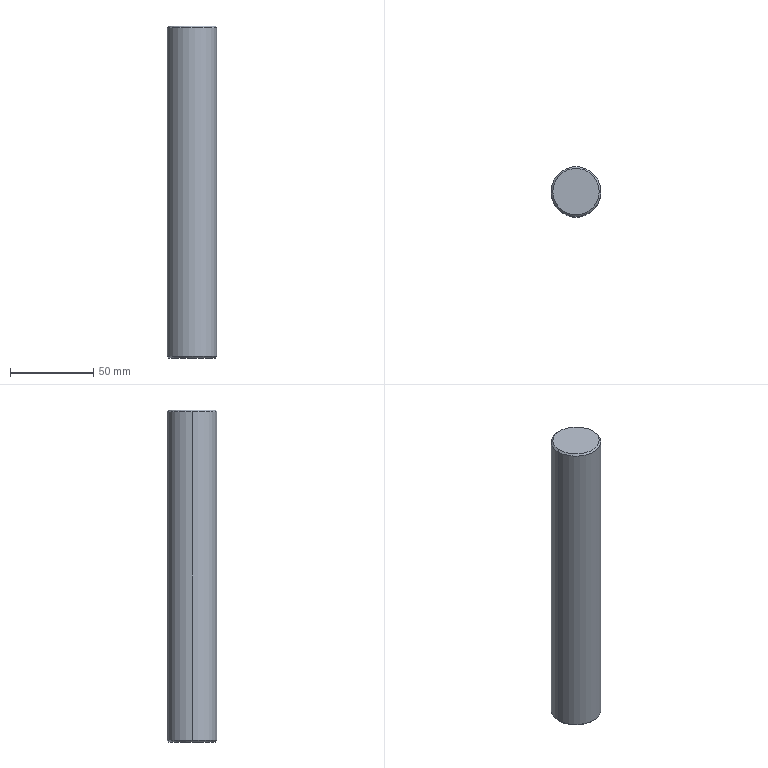Part | SolidWorks | 1 solid | 8 faces | box 30 x 30 x 200 mm | volume 141280 mm3 | cone 4 | cylinder 2 | plane 2 | commonest cylinder face diameters 30 x2
STEP:
#1=CARTESIAN_POINT('',(14.,0.,200.));
#2=VERTEX_POINT('',#1);
#3=CARTESIAN_POINT('',(-14.,0.,200.));
#4=VERTEX_POINT('',#3);
#5=CARTESIAN_POINT('',(0.,0.,200.));
#6=DIRECTION('',(0.,0.,1.));
#7=DIRECTION('',(1.,0.,0.));
#8=AXIS2_PLACEMENT_3D('',#5,#6,#7);
#9=CIRCLE('',#8,14.);
#10=EDGE_CURVE('',#2,#4,#9,.T.);
#11=ORIENTED_EDGE('',*,*,#10,.F.);
#12=CARTESIAN_POINT('',(15.,0.,199.));
#13=VERTEX_POINT('',#12);
#14=CARTESIAN_POINT('',(14.,0.,200.));
#15=DIRECTION('',(0.7071,0.,-0.7071));
#16=VECTOR('',#15,1000.);
#17=LINE('',#14,#16);
#18=EDGE_CURVE('',#2,#13,#17,.T.);
#19=ORIENTED_EDGE('',*,*,#18,.T.);
#20=CARTESIAN_POINT('',(-15.,0.,199.));
#21=VERTEX_POINT('',#20);
#22=CARTESIAN_POINT('',(0.,0.,199.));
#23=DIRECTION('',(0.,0.,-1.));
#24=DIRECTION('',(1.,0.,0.));
#25=AXIS2_PLACEMENT_3D('',#22,#23,#24);
#26=CIRCLE('',#25,15.);
#27=EDGE_CURVE('',#21,#13,#26,.T.);
#28=ORIENTED_EDGE('',*,*,#27,.F.);
#29=CARTESIAN_POINT('',(-14.,0.,200.));
#30=DIRECTION('',(-0.7071,0.,-0.7071));
#31=VECTOR('',#30,1000.);
#32=LINE('',#29,#31);
#33=EDGE_CURVE('',#4,#21,#32,.T.);
#34=ORIENTED_EDGE('',*,*,#33,.F.);
#35=EDGE_LOOP('',(#11,#19,#28,#34));
#36=FACE_OUTER_BOUND('',#35,.T.);
#37=CARTESIAN_POINT('',(0.,0.,200.));
#38=DIRECTION('',(0.,0.,-1.));
#39=DIRECTION('',(-1.,0.,0.));
#40=AXIS2_PLACEMENT_3D('',#37,#38,#39);
#41=CONICAL_SURFACE('',#40,14.,0.7854);
#42=ADVANCED_FACE('',(#36),#41,.T.);
#43=CARTESIAN_POINT('',(-14.,0.,0.));
#44=VERTEX_POINT('',#43);
#45=CARTESIAN_POINT('',(14.,0.,0.));
#46=VERTEX_POINT('',#45);
#47=CARTESIAN_POINT('',(0.,0.,0.));
#48=DIRECTION('',(0.,0.,-1.));
#49=DIRECTION('',(1.,0.,0.));
#50=AXIS2_PLACEMENT_3D('',#47,#48,#49);
#51=CIRCLE('',#50,14.);
#52=EDGE_CURVE('',#44,#46,#51,.T.);
#53=ORIENTED_EDGE('',*,*,#52,.F.);
#54=CARTESIAN_POINT('',(-15.,0.,1.));
#55=VERTEX_POINT('',#54);
#56=CARTESIAN_POINT('',(-15.,0.,1.));
#57=DIRECTION('',(-0.7071,0.,0.7071));
#58=VECTOR('',#57,1000.);
#59=LINE('',#56,#58);
#60=EDGE_CURVE('',#44,#55,#59,.T.);
#61=ORIENTED_EDGE('',*,*,#60,.T.);
#62=CARTESIAN_POINT('',(15.,0.,1.));
#63=VERTEX_POINT('',#62);
#64=CARTESIAN_POINT('',(0.,0.,1.));
#65=DIRECTION('',(0.,0.,1.));
#66=DIRECTION('',(1.,0.,0.));
#67=AXIS2_PLACEMENT_3D('',#64,#65,#66);
#68=CIRCLE('',#67,15.);
#69=EDGE_CURVE('',#63,#55,#68,.T.);
#70=ORIENTED_EDGE('',*,*,#69,.F.);
#71=CARTESIAN_POINT('',(15.,0.,1.));
#72=DIRECTION('',(0.7071,0.,0.7071));
#73=VECTOR('',#72,1000.);
#74=LINE('',#71,#73);
#75=EDGE_CURVE('',#46,#63,#74,.T.);
#76=ORIENTED_EDGE('',*,*,#75,.F.);
#77=EDGE_LOOP('',(#53,#61,#70,#76));
#78=FACE_OUTER_BOUND('',#77,.T.);
#79=CARTESIAN_POINT('',(0.,0.,1.));
#80=DIRECTION('',(0.,0.,1.));
#81=DIRECTION('',(1.,0.,0.));
#82=AXIS2_PLACEMENT_3D('',#79,#80,#81);
#83=CONICAL_SURFACE('',#82,15.,0.7854);
#84=ADVANCED_FACE('',(#78),#83,.T.);
#85=ORIENTED_EDGE('',*,*,#27,.T.);
#86=CARTESIAN_POINT('',(15.,0.,200.));
#87=DIRECTION('',(0.,0.,-1.));
#88=VECTOR('',#87,1000.);
#89=LINE('',#86,#88);
#90=EDGE_CURVE('',#13,#63,#89,.T.);
#91=ORIENTED_EDGE('',*,*,#90,.T.);
#92=ORIENTED_EDGE('',*,*,#69,.T.);
#93=CARTESIAN_POINT('',(-15.,0.,200.));
#94=DIRECTION('',(0.,0.,-1.));
#95=VECTOR('',#94,1000.);
#96=LINE('',#93,#95);
#97=EDGE_CURVE('',#21,#55,#96,.T.);
#98=ORIENTED_EDGE('',*,*,#97,.F.);
#99=EDGE_LOOP('',(#85,#91,#92,#98));
#100=FACE_OUTER_BOUND('',#99,.T.);
#101=CARTESIAN_POINT('',(0.,0.,200.));
#102=DIRECTION('',(0.,0.,-1.));
#103=DIRECTION('',(-1.,0.,0.));
#104=AXIS2_PLACEMENT_3D('',#101,#102,#103);
#105=CYLINDRICAL_SURFACE('',#104,15.);
#106=ADVANCED_FACE('',(#100),#105,.T.);
#107=ORIENTED_EDGE('',*,*,#90,.F.);
#108=CARTESIAN_POINT('',(0.,0.,199.));
#109=DIRECTION('',(0.,0.,-1.));
#110=DIRECTION('',(1.,0.,0.));
#111=AXIS2_PLACEMENT_3D('',#108,#109,#110);
#112=CIRCLE('',#111,15.);
#113=EDGE_CURVE('',#13,#21,#112,.T.);
#114=ORIENTED_EDGE('',*,*,#113,.T.);
#115=ORIENTED_EDGE('',*,*,#97,.T.);
#116=CARTESIAN_POINT('',(0.,0.,1.));
#117=DIRECTION('',(0.,0.,1.));
#118=DIRECTION('',(1.,0.,0.));
#119=AXIS2_PLACEMENT_3D('',#116,#117,#118);
#120=CIRCLE('',#119,15.);
#121=EDGE_CURVE('',#55,#63,#120,.T.);
#122=ORIENTED_EDGE('',*,*,#121,.T.);
#123=EDGE_LOOP('',(#107,#114,#115,#122));
#124=FACE_OUTER_BOUND('',#123,.T.);
#125=CARTESIAN_POINT('',(0.,0.,200.));
#126=DIRECTION('',(0.,0.,-1.));
#127=DIRECTION('',(-1.,0.,0.));
#128=AXIS2_PLACEMENT_3D('',#125,#126,#127);
#129=CYLINDRICAL_SURFACE('',#128,15.);
#130=ADVANCED_FACE('',(#124),#129,.T.);
#131=CARTESIAN_POINT('',(0.,0.,200.));
#132=DIRECTION('',(0.,0.,1.));
#133=DIRECTION('',(1.,0.,0.));
#134=AXIS2_PLACEMENT_3D('',#131,#132,#133);
#135=CIRCLE('',#134,14.);
#136=EDGE_CURVE('',#4,#2,#135,.T.);
#137=ORIENTED_EDGE('',*,*,#136,.T.);
#138=ORIENTED_EDGE('',*,*,#10,.T.);
#139=EDGE_LOOP('',(#137,#138));
#140=FACE_OUTER_BOUND('',#139,.T.);
#141=CARTESIAN_POINT('',(0.,0.,200.));
#142=DIRECTION('',(0.,0.,1.));
#143=DIRECTION('',(1.,0.,0.));
#144=AXIS2_PLACEMENT_3D('',#141,#142,#143);
#145=PLANE('',#144);
#146=ADVANCED_FACE('',(#140),#145,.T.);
#147=CARTESIAN_POINT('',(0.,0.,0.));
#148=DIRECTION('',(0.,0.,-1.));
#149=DIRECTION('',(1.,0.,0.));
#150=AXIS2_PLACEMENT_3D('',#147,#148,#149);
#151=CIRCLE('',#150,14.);
#152=EDGE_CURVE('',#46,#44,#151,.T.);
#153=ORIENTED_EDGE('',*,*,#152,.T.);
#154=ORIENTED_EDGE('',*,*,#52,.T.);
#155=EDGE_LOOP('',(#153,#154));
#156=FACE_OUTER_BOUND('',#155,.T.);
#157=CARTESIAN_POINT('',(0.,0.,0.));
#158=DIRECTION('',(0.,0.,1.));
#159=DIRECTION('',(1.,0.,0.));
#160=AXIS2_PLACEMENT_3D('',#157,#158,#159);
#161=PLANE('',#160);
#162=ADVANCED_FACE('',(#156),#161,.F.);
#163=ORIENTED_EDGE('',*,*,#60,.F.);
#164=ORIENTED_EDGE('',*,*,#152,.F.);
#165=ORIENTED_EDGE('',*,*,#75,.T.);
#166=ORIENTED_EDGE('',*,*,#121,.F.);
#167=EDGE_LOOP('',(#163,#164,#165,#166));
#168=FACE_OUTER_BOUND('',#167,.T.);
#169=CARTESIAN_POINT('',(0.,0.,1.));
#170=DIRECTION('',(0.,0.,1.));
#171=DIRECTION('',(1.,0.,0.));
#172=AXIS2_PLACEMENT_3D('',#169,#170,#171);
#173=CONICAL_SURFACE('',#172,15.,0.7854);
#174=ADVANCED_FACE('',(#168),#173,.T.);
#175=ORIENTED_EDGE('',*,*,#18,.F.);
#176=ORIENTED_EDGE('',*,*,#136,.F.);
#177=ORIENTED_EDGE('',*,*,#33,.T.);
#178=ORIENTED_EDGE('',*,*,#113,.F.);
#179=EDGE_LOOP('',(#175,#176,#177,#178));
#180=FACE_OUTER_BOUND('',#179,.T.);
#181=CARTESIAN_POINT('',(0.,0.,200.));
#182=DIRECTION('',(0.,0.,-1.));
#183=DIRECTION('',(-1.,0.,0.));
#184=AXIS2_PLACEMENT_3D('',#181,#182,#183);
#185=CONICAL_SURFACE('',#184,14.,0.7854);
#186=ADVANCED_FACE('',(#180),#185,.T.);
#187=CLOSED_SHELL('',(#42,#84,#106,#130,#146,#162,#174,#186));
#188=MANIFOLD_SOLID_BREP('',#187);
#189=CARTESIAN_POINT('',(0.,0.,0.));
#190=DIRECTION('',(0.,0.,1.));
#191=DIRECTION('',(1.,0.,0.));
#192=AXIS2_PLACEMENT_3D('',#189,#190,#191);
#193=(LENGTH_UNIT()NAMED_UNIT(*)SI_UNIT(.MILLI.,.METRE.));
#194=UNCERTAINTY_MEASURE_WITH_UNIT(LENGTH_MEASURE(0.00001),#193,'','');
#195=(NAMED_UNIT(*)PLANE_ANGLE_UNIT()SI_UNIT($,.RADIAN.));
#196=(NAMED_UNIT(*)SI_UNIT($,.STERADIAN.)SOLID_ANGLE_UNIT());
#197=(GEOMETRIC_REPRESENTATION_CONTEXT(3)GLOBAL_UNCERTAINTY_ASSIGNED_CONTEXT((#194))GLOBAL_UNIT_ASSIGNED_CONTEXT((#193,#195,#196))REPRESENTATION_CONTEXT('',''));
#198=ADVANCED_BREP_SHAPE_REPRESENTATION('',(#188,#192),#197);